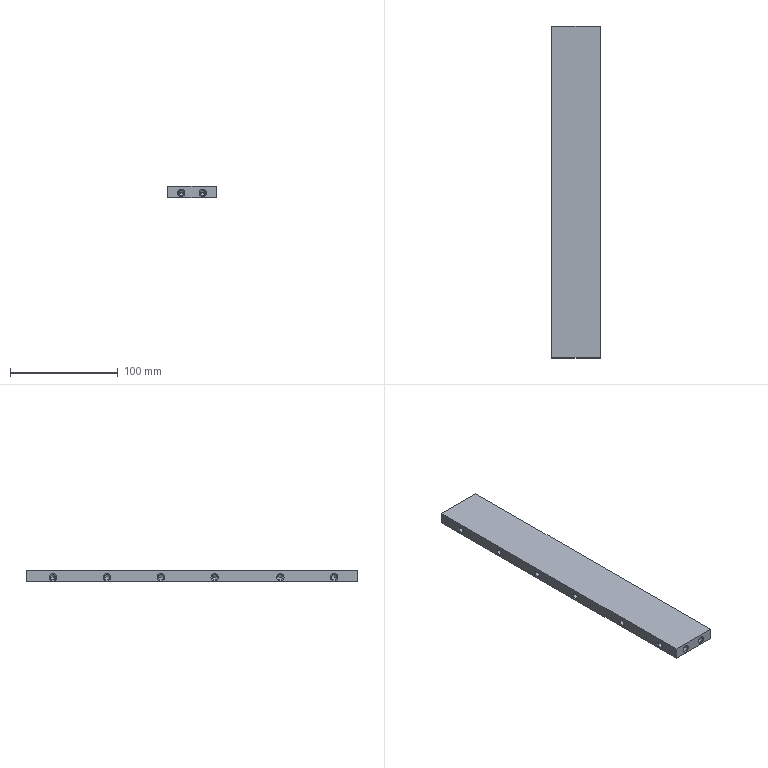Part | NX | 1 solid | 90 faces | box 45 x 308 x 10.5 mm | volume 140655 mm3 | cone 56 | cylinder 28 | plane 6 | commonest cylinder face diameters 5 x28